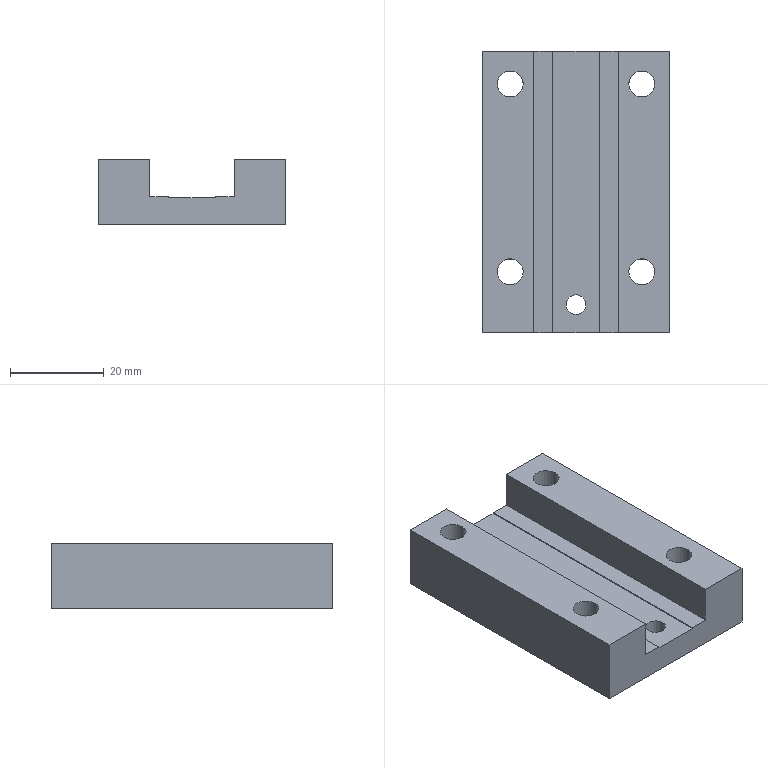Part | STEP file | BU-C06-2 | 1 solid | 24 faces | box 40 x 60 x 14 mm | volume 23429 mm3 | plane 14 | cylinder 10 | commonest cylinder face diameters 5.5 x8 4.2 x2